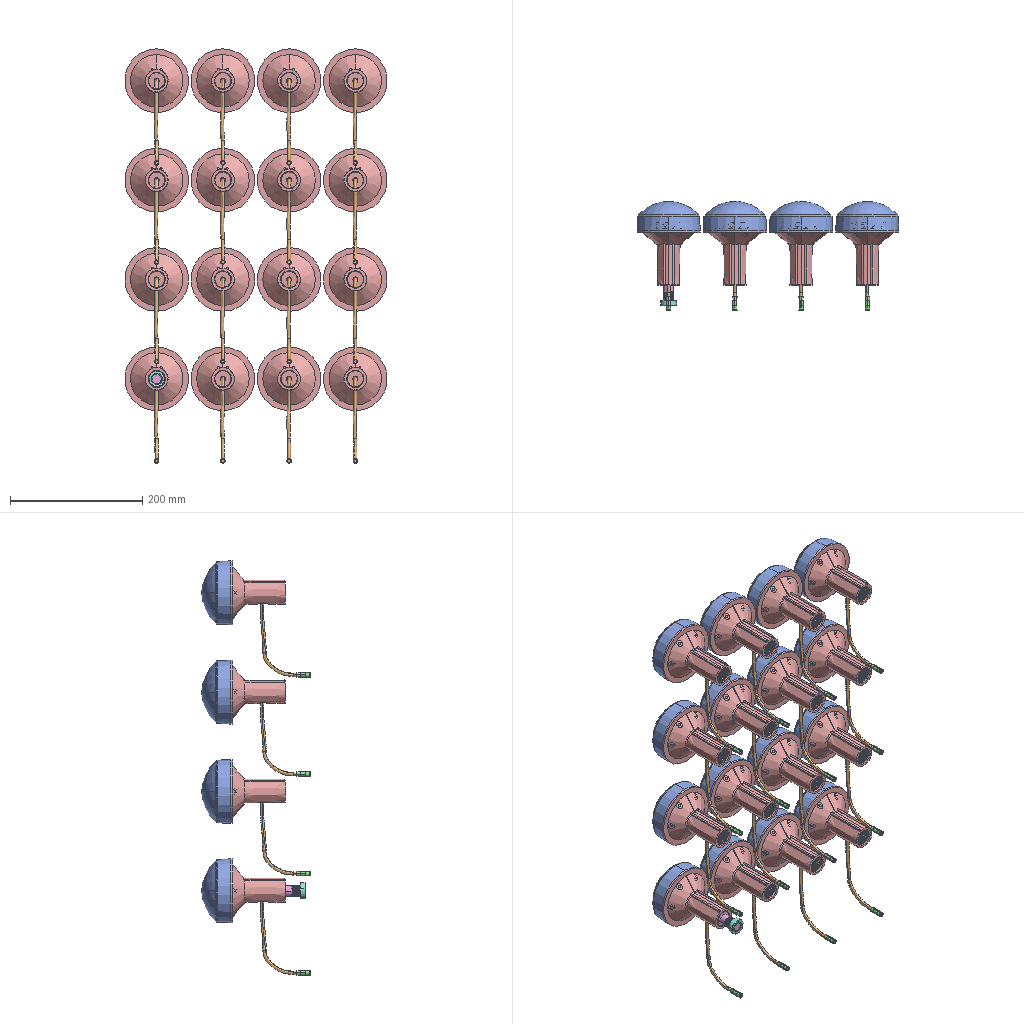Assembly | SolidWorks | 12 different items | 180 placed | box 396 x 164 x 626 mm
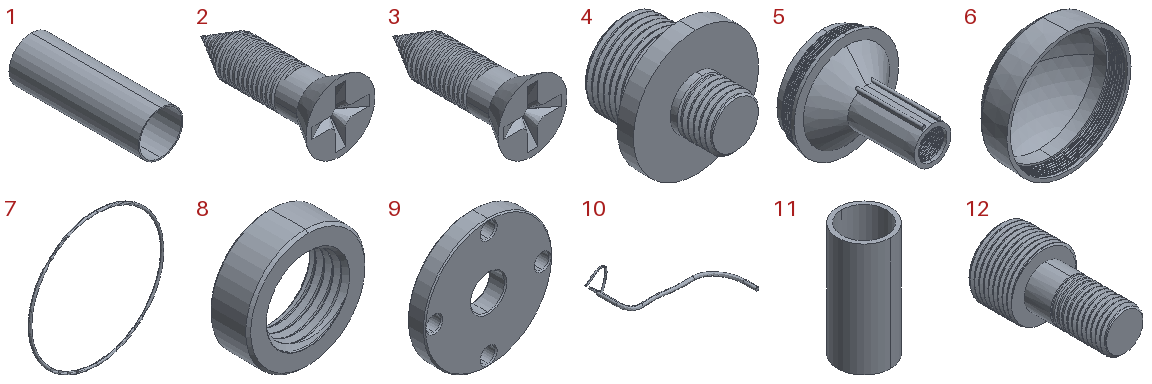Parts list (item | quantity | size | volume | features):
1 | x16 | 6.9 x 20 x 6.9 mm | 84.195 mm3 | features ExtruThin 1
2 | x64 | 5.2 x 10.5 x 5.2 mm | 67.225 mm3 | features BlendCut 1, Helix 1, ICE 1, Revolution 1, SweepCut 1
3 | x1 | 5.2 x 10.5 x 5.2 mm | 67.225 mm3 | features BlendCut 1, Helix 1, ICE 1, Revolution 1, SweepCut 1
4 | x1 | 38 x 34 x 38 mm | 15399 mm3 | features Helix 2, SweepCut 2, Revolution 1
5 | x16 | 96.5 x 101.609 x 96.5 mm | 64001 mm3 | features ICE 6, Helix 2, SweepCut 2, Revolution 1
6 | x16 | 96.5 x 43.5 x 96.5 mm | 37980 mm3 | features Helix 1, Revolution 1, SweepCut 1
7 | x16 | 87.4 x 1.7 x 87.4 mm | 611.109 mm3 | features Revolution 1
8 | x1 | 24 x 8 x 24 mm | 1989 mm3 | features Chamfer 2, Extrusion 1, Helix 1, SweepCut 1
9 | x16 | 22.5 x 3 x 22.5 mm | 1039 mm3 | features Chamfer 1, Extrusion 1
10 | x16 | 128.902 x 134.039 x 36.156 mm | 4687 mm3 | features 3DProfileFeature 4, Sweep 2
11 | x16 | 6.3 x 6.3 x 13.5 mm | 122.993 mm3 | features Revolution 1
12 | x1 | 25.2 x 47 x 25.2 mm | 13171 mm3 | features Helix 2, SweepCut 2, Revolution 1
Mates (type | each side: item.copy, entity, surface, feature):
Coordinate | 5.1 select_type:25 | assembly select_type:11
Coincident | 5.1 face cylinder Revolve1 | 6.1 edge
Coincident | 5.1 face plane Revolve1 | 6.1 face plane Revolve1
Coincident | 5.1 axis | 7.1 axis
Tangent | 5.1 face plane Revolve1 | 7.1 face torus Revolve1
Concentric | 5.1 face cone Revolve1 | 12.1 face cylinder Revolve1
Coincident | 5.1 face plane Revolve1 | 12.1 face plane Revolve1
Coincident | 5.1 plane | 10.1 plane
Concentric | 5.1 face cylinder Revolve1 | 10.1 face cylinder Sweep2
DistanceDim | 10.1 face plane Sweep2 | 5.1 face plane Revolve1
Concentric | 10.1 face cylinder Sweep2 | 11.1 face cylinder Revolve1
Concentric | 11.1 face cylinder Revolve1 | 1.1 face cylinder Extrude-Thin1
Coincident | 5.1 face plane Revolve1 | 9.1 face plane Boss-Extrude1
Concentric | 5.1 face cylinder Cut-Extrude3 | 9.1 face cylinder Boss-Extrude1 | 2 times
Concentric | 9.1 face cylinder Boss-Extrude1 | 2.1 edge
DistanceDim | 2.1 face plane Revolve2 | 9.1 face plane Boss-Extrude1
DistanceDim | 2.2 face plane Revolve2 | 9.1 face plane Boss-Extrude1
Concentric | 9.1 edge | 2.2 edge
Concentric | 9.1 face cylinder Boss-Extrude1 | 2.3 edge
DistanceDim | 2.3 face plane Revolve2 | 9.1 face plane Boss-Extrude1
Concentric | 9.1 face cylinder Boss-Extrude1 | 2.4 edge
DistanceDim | 2.4 face plane Revolve2 | 9.1 face plane Boss-Extrude1